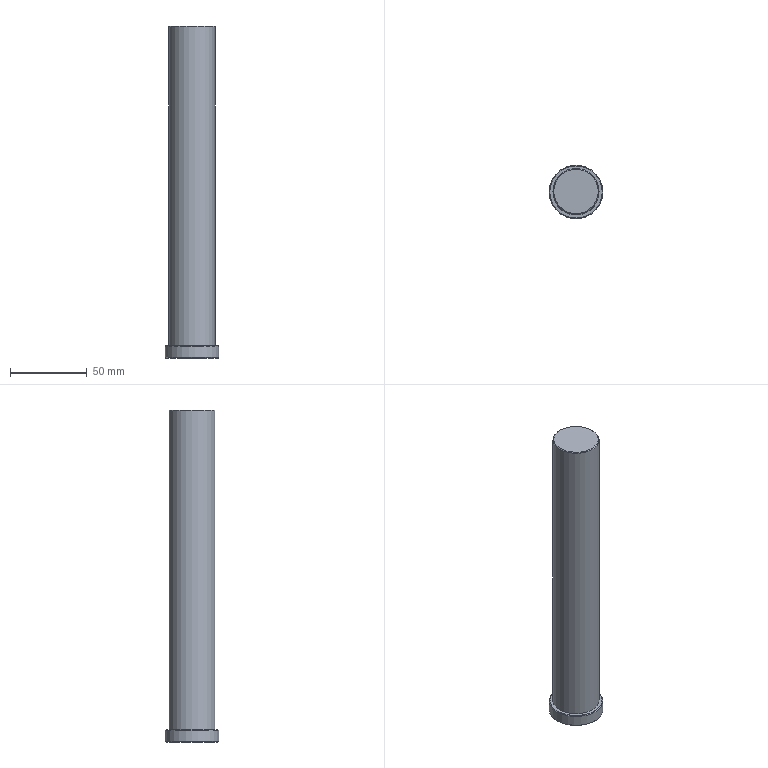Part | NX | features 模具.stp<1>[35] 2 | 1 solid | 8 faces | box 35 x 35 x 216 mm | volume 154685 mm3 | cone 3 | plane 3 | cylinder 2 | commonest cylinder face diameters 30 x1 35 x1
STEP:
#1=CARTESIAN_POINT('',(175.,-315.,0.));
#2=VERTEX_POINT('',#1);
#3=CARTESIAN_POINT('',(160.,-315.,0.));
#4=DIRECTION('',(0.,0.,-1.));
#5=DIRECTION('',(1.,0.,0.));
#6=AXIS2_PLACEMENT_3D('',#3,#4,#5);
#7=CIRCLE('',#6,15.);
#8=EDGE_CURVE('',#2,#2,#7,.T.);
#9=ORIENTED_EDGE('',*,*,#8,.F.);
#10=EDGE_LOOP('',(#9));
#11=FACE_BOUND('',#10,.T.);
#12=CARTESIAN_POINT('',(174.5,-315.,0.5));
#13=VERTEX_POINT('',#12);
#14=CARTESIAN_POINT('',(160.,-315.,0.5));
#15=DIRECTION('',(0.,0.,1.));
#16=DIRECTION('',(1.,0.,0.));
#17=AXIS2_PLACEMENT_3D('',#14,#15,#16);
#18=CIRCLE('',#17,14.5);
#19=EDGE_CURVE('',#13,#13,#18,.T.);
#20=ORIENTED_EDGE('',*,*,#19,.F.);
#21=EDGE_LOOP('',(#20));
#22=FACE_BOUND('',#21,.T.);
#23=CARTESIAN_POINT('',(160.,-315.,0.));
#24=DIRECTION('',(0.,0.,-1.));
#25=DIRECTION('',(-1.,0.,0.));
#26=AXIS2_PLACEMENT_3D('',#23,#24,#25);
#27=CONICAL_SURFACE('',#26,15.,0.7854);
#28=ADVANCED_FACE('',(#11,#22),#27,.T.);
#29=ORIENTED_EDGE('',*,*,#8,.T.);
#30=EDGE_LOOP('',(#29));
#31=FACE_BOUND('',#30,.T.);
#32=CARTESIAN_POINT('',(175.,-315.,-207.5));
#33=VERTEX_POINT('',#32);
#34=CARTESIAN_POINT('',(160.,-315.,-207.5));
#35=DIRECTION('',(0.,0.,1.));
#36=DIRECTION('',(1.,0.,0.));
#37=AXIS2_PLACEMENT_3D('',#34,#35,#36);
#38=CIRCLE('',#37,15.);
#39=EDGE_CURVE('',#33,#33,#38,.T.);
#40=ORIENTED_EDGE('',*,*,#39,.T.);
#41=EDGE_LOOP('',(#40));
#42=FACE_BOUND('',#41,.T.);
#43=CARTESIAN_POINT('',(160.,-315.,-215.5));
#44=DIRECTION('',(0.,0.,1.));
#45=DIRECTION('',(1.,0.,0.));
#46=AXIS2_PLACEMENT_3D('',#43,#44,#45);
#47=CYLINDRICAL_SURFACE('',#46,15.);
#48=ADVANCED_FACE('',(#31,#42),#47,.T.);
#49=ORIENTED_EDGE('',*,*,#19,.T.);
#50=EDGE_LOOP('',(#49));
#51=FACE_BOUND('',#50,.T.);
#52=CARTESIAN_POINT('',(160.,-315.,0.5));
#53=DIRECTION('',(0.,0.,1.));
#54=DIRECTION('',(1.,0.,0.));
#55=AXIS2_PLACEMENT_3D('',#52,#53,#54);
#56=PLANE('',#55);
#57=ADVANCED_FACE('',(#51),#56,.T.);
#58=CARTESIAN_POINT('',(177.5,-315.,-208.));
#59=VERTEX_POINT('',#58);
#60=CARTESIAN_POINT('',(160.,-315.,-208.));
#61=DIRECTION('',(0.,0.,-1.));
#62=DIRECTION('',(1.,0.,0.));
#63=AXIS2_PLACEMENT_3D('',#60,#61,#62);
#64=CIRCLE('',#63,17.5);
#65=EDGE_CURVE('',#59,#59,#64,.T.);
#66=ORIENTED_EDGE('',*,*,#65,.F.);
#67=EDGE_LOOP('',(#66));
#68=FACE_BOUND('',#67,.T.);
#69=CARTESIAN_POINT('',(177.,-315.,-207.5));
#70=VERTEX_POINT('',#69);
#71=CARTESIAN_POINT('',(160.,-315.,-207.5));
#72=DIRECTION('',(0.,0.,1.));
#73=DIRECTION('',(1.,0.,0.));
#74=AXIS2_PLACEMENT_3D('',#71,#72,#73);
#75=CIRCLE('',#74,17.);
#76=EDGE_CURVE('',#70,#70,#75,.T.);
#77=ORIENTED_EDGE('',*,*,#76,.F.);
#78=EDGE_LOOP('',(#77));
#79=FACE_BOUND('',#78,.T.);
#80=CARTESIAN_POINT('',(160.,-315.,-208.));
#81=DIRECTION('',(0.,0.,-1.));
#82=DIRECTION('',(-1.,0.,0.));
#83=AXIS2_PLACEMENT_3D('',#80,#81,#82);
#84=CONICAL_SURFACE('',#83,17.5,0.7854);
#85=ADVANCED_FACE('',(#68,#79),#84,.T.);
#86=CARTESIAN_POINT('',(142.5,-315.,-215.));
#87=VERTEX_POINT('',#86);
#88=CARTESIAN_POINT('',(160.,-315.,-215.));
#89=DIRECTION('',(0.,0.,1.));
#90=DIRECTION('',(-1.,0.,0.));
#91=AXIS2_PLACEMENT_3D('',#88,#89,#90);
#92=CIRCLE('',#91,17.5);
#93=EDGE_CURVE('',#87,#87,#92,.T.);
#94=ORIENTED_EDGE('',*,*,#93,.F.);
#95=EDGE_LOOP('',(#94));
#96=FACE_BOUND('',#95,.T.);
#97=CARTESIAN_POINT('',(143.,-315.,-215.5));
#98=VERTEX_POINT('',#97);
#99=CARTESIAN_POINT('',(160.,-315.,-215.5));
#100=DIRECTION('',(0.,0.,-1.));
#101=DIRECTION('',(-1.,0.,0.));
#102=AXIS2_PLACEMENT_3D('',#99,#100,#101);
#103=CIRCLE('',#102,17.);
#104=EDGE_CURVE('',#98,#98,#103,.T.);
#105=ORIENTED_EDGE('',*,*,#104,.F.);
#106=EDGE_LOOP('',(#105));
#107=FACE_BOUND('',#106,.T.);
#108=CARTESIAN_POINT('',(160.,-315.,-215.));
#109=DIRECTION('',(0.,0.,1.));
#110=DIRECTION('',(1.,0.,0.));
#111=AXIS2_PLACEMENT_3D('',#108,#109,#110);
#112=CONICAL_SURFACE('',#111,17.5,0.7854);
#113=ADVANCED_FACE('',(#96,#107),#112,.T.);
#114=ORIENTED_EDGE('',*,*,#65,.T.);
#115=EDGE_LOOP('',(#114));
#116=FACE_BOUND('',#115,.T.);
#117=ORIENTED_EDGE('',*,*,#93,.T.);
#118=EDGE_LOOP('',(#117));
#119=FACE_BOUND('',#118,.T.);
#120=CARTESIAN_POINT('',(160.,-315.,-215.5));
#121=DIRECTION('',(0.,0.,1.));
#122=DIRECTION('',(1.,0.,0.));
#123=AXIS2_PLACEMENT_3D('',#120,#121,#122);
#124=CYLINDRICAL_SURFACE('',#123,17.5);
#125=ADVANCED_FACE('',(#116,#119),#124,.T.);
#126=ORIENTED_EDGE('',*,*,#104,.T.);
#127=EDGE_LOOP('',(#126));
#128=FACE_BOUND('',#127,.T.);
#129=CARTESIAN_POINT('',(160.,-315.,-215.5));
#130=DIRECTION('',(0.,0.,-1.));
#131=DIRECTION('',(0.,-1.,0.));
#132=AXIS2_PLACEMENT_3D('',#129,#130,#131);
#133=PLANE('',#132);
#134=ADVANCED_FACE('',(#128),#133,.T.);
#135=ORIENTED_EDGE('',*,*,#76,.T.);
#136=EDGE_LOOP('',(#135));
#137=FACE_BOUND('',#136,.T.);
#138=ORIENTED_EDGE('',*,*,#39,.F.);
#139=EDGE_LOOP('',(#138));
#140=FACE_BOUND('',#139,.T.);
#141=CARTESIAN_POINT('',(160.,-315.,-207.5));
#142=DIRECTION('',(0.,0.,1.));
#143=DIRECTION('',(1.,0.,0.));
#144=AXIS2_PLACEMENT_3D('',#141,#142,#143);
#145=PLANE('',#144);
#146=ADVANCED_FACE('',(#137,#140),#145,.T.);
#147=CLOSED_SHELL('',(#28,#48,#57,#85,#113,#125,#134,#146));
#148=MANIFOLD_SOLID_BREP('',#147);
#149=(LENGTH_UNIT()NAMED_UNIT(*)SI_UNIT(.MILLI.,.METRE.));
#150=UNCERTAINTY_MEASURE_WITH_UNIT(LENGTH_MEASURE(0.00001),#149,'','');
#151=(NAMED_UNIT(*)PLANE_ANGLE_UNIT()SI_UNIT($,.RADIAN.));
#152=(NAMED_UNIT(*)SI_UNIT($,.STERADIAN.)SOLID_ANGLE_UNIT());
#153=(GEOMETRIC_REPRESENTATION_CONTEXT(3)GLOBAL_UNCERTAINTY_ASSIGNED_CONTEXT((#150))GLOBAL_UNIT_ASSIGNED_CONTEXT((#149,#151,#152))REPRESENTATION_CONTEXT('',''));
#154=ADVANCED_BREP_SHAPE_REPRESENTATION('',(#148),#153);